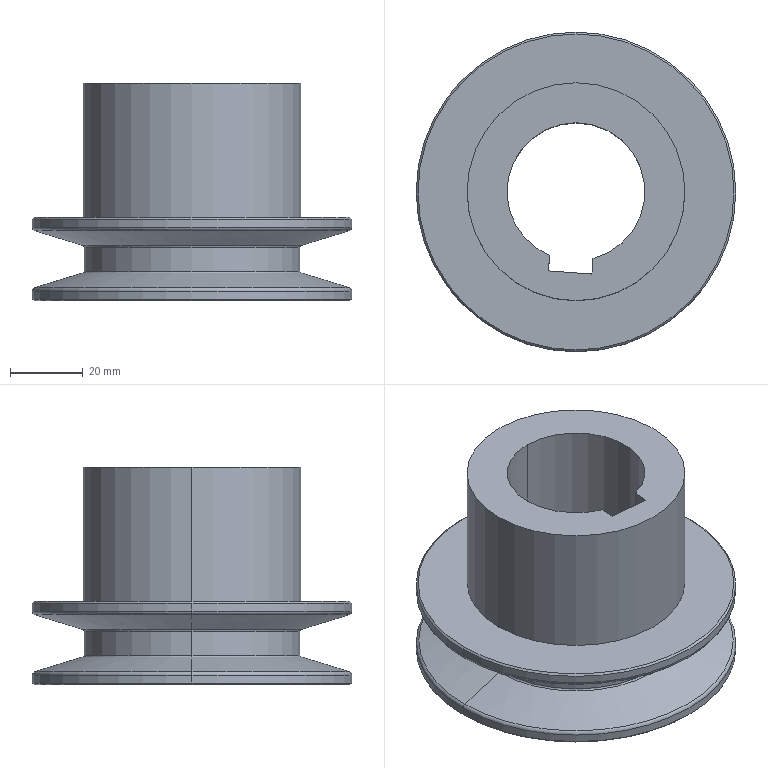Part | SolidWorks | features Fillet 2, ICE 2, Chamfer 1, RevCut 1, Revolution 1 | 1 solid | 32 faces | box 88 x 88 x 60 mm | volume 133834 mm3 | cylinder 10 | torus 8 | cone 8 | plane 6 | commonest cylinder face diameters 88 x4 38 x2 59.4 x2 60 x2
STEP:
#1=CARTESIAN_POINT('',(619.523,22.744,-118.047));
#2=VERTEX_POINT('',#1);
#3=CARTESIAN_POINT('',(532.938,22.744,-118.047));
#4=VERTEX_POINT('',#3);
#5=CARTESIAN_POINT('',(576.231,22.744,-118.047));
#6=DIRECTION('',(0.,0.,1.));
#7=DIRECTION('',(1.,0.,0.));
#8=AXIS2_PLACEMENT_3D('',#5,#6,#7);
#9=CIRCLE('',#8,43.292);
#10=EDGE_CURVE('',#2,#4,#9,.T.);
#11=ORIENTED_EDGE('',*,*,#10,.F.);
#12=CARTESIAN_POINT('',(620.231,22.744,-119.003));
#13=VERTEX_POINT('',#12);
#14=CARTESIAN_POINT('',(619.231,22.744,-119.003));
#15=DIRECTION('',(0.,1.,0.));
#16=DIRECTION('',(-1.,0.,0.));
#17=AXIS2_PLACEMENT_3D('',#14,#15,#16);
#18=CIRCLE('',#17,1.);
#19=EDGE_CURVE('',#2,#13,#18,.T.);
#20=ORIENTED_EDGE('',*,*,#19,.T.);
#21=CARTESIAN_POINT('',(532.231,22.744,-119.003));
#22=VERTEX_POINT('',#21);
#23=CARTESIAN_POINT('',(576.231,22.744,-119.003));
#24=DIRECTION('',(0.,0.,-1.));
#25=DIRECTION('',(-1.,0.,0.));
#26=AXIS2_PLACEMENT_3D('',#23,#24,#25);
#27=CIRCLE('',#26,44.);
#28=EDGE_CURVE('',#22,#13,#27,.T.);
#29=ORIENTED_EDGE('',*,*,#28,.F.);
#30=CARTESIAN_POINT('',(533.231,22.744,-119.003));
#31=DIRECTION('',(0.,-1.,0.));
#32=DIRECTION('',(0.,0.,-1.));
#33=AXIS2_PLACEMENT_3D('',#30,#31,#32);
#34=CIRCLE('',#33,1.);
#35=EDGE_CURVE('',#4,#22,#34,.T.);
#36=ORIENTED_EDGE('',*,*,#35,.F.);
#37=EDGE_LOOP('',(#11,#20,#29,#36));
#38=FACE_OUTER_BOUND('',#37,.T.);
#39=CARTESIAN_POINT('',(576.231,22.744,-119.003));
#40=DIRECTION('',(0.,0.,-1.));
#41=DIRECTION('',(-1.,0.,0.));
#42=AXIS2_PLACEMENT_3D('',#39,#40,#41);
#43=TOROIDAL_SURFACE('',#42,43.,1.);
#44=ADVANCED_FACE('',(#38),#43,.T.);
#45=CARTESIAN_POINT('',(620.231,22.744,-101.383));
#46=VERTEX_POINT('',#45);
#47=CARTESIAN_POINT('',(532.231,22.744,-101.383));
#48=VERTEX_POINT('',#47);
#49=CARTESIAN_POINT('',(576.231,22.744,-101.383));
#50=DIRECTION('',(0.,0.,1.));
#51=DIRECTION('',(-1.,0.,0.));
#52=AXIS2_PLACEMENT_3D('',#49,#50,#51);
#53=CIRCLE('',#52,44.);
#54=EDGE_CURVE('',#46,#48,#53,.T.);
#55=ORIENTED_EDGE('',*,*,#54,.F.);
#56=CARTESIAN_POINT('',(619.523,22.744,-102.339));
#57=VERTEX_POINT('',#56);
#58=CARTESIAN_POINT('',(619.231,22.744,-101.383));
#59=DIRECTION('',(0.,1.,0.));
#60=DIRECTION('',(-1.,0.,0.));
#61=AXIS2_PLACEMENT_3D('',#58,#59,#60);
#62=CIRCLE('',#61,1.);
#63=EDGE_CURVE('',#46,#57,#62,.T.);
#64=ORIENTED_EDGE('',*,*,#63,.T.);
#65=CARTESIAN_POINT('',(532.938,22.744,-102.339));
#66=VERTEX_POINT('',#65);
#67=CARTESIAN_POINT('',(576.231,22.744,-102.339));
#68=DIRECTION('',(0.,0.,-1.));
#69=DIRECTION('',(-1.,0.,0.));
#70=AXIS2_PLACEMENT_3D('',#67,#68,#69);
#71=CIRCLE('',#70,43.292);
#72=EDGE_CURVE('',#66,#57,#71,.T.);
#73=ORIENTED_EDGE('',*,*,#72,.F.);
#74=CARTESIAN_POINT('',(533.231,22.744,-101.383));
#75=DIRECTION('',(0.,-1.,0.));
#76=DIRECTION('',(0.,0.,-1.));
#77=AXIS2_PLACEMENT_3D('',#74,#75,#76);
#78=CIRCLE('',#77,1.);
#79=EDGE_CURVE('',#48,#66,#78,.T.);
#80=ORIENTED_EDGE('',*,*,#79,.F.);
#81=EDGE_LOOP('',(#55,#64,#73,#80));
#82=FACE_OUTER_BOUND('',#81,.T.);
#83=CARTESIAN_POINT('',(576.231,22.744,-101.383));
#84=DIRECTION('',(0.,0.,-1.));
#85=DIRECTION('',(-1.,0.,0.));
#86=AXIS2_PLACEMENT_3D('',#83,#84,#85);
#87=TOROIDAL_SURFACE('',#86,43.,1.);
#88=ADVANCED_FACE('',(#82),#87,.T.);
#89=CARTESIAN_POINT('',(546.531,22.744,-113.521));
#90=VERTEX_POINT('',#89);
#91=CARTESIAN_POINT('',(605.931,22.744,-113.521));
#92=VERTEX_POINT('',#91);
#93=CARTESIAN_POINT('',(576.231,22.744,-113.521));
#94=DIRECTION('',(0.,0.,1.));
#95=DIRECTION('',(1.,0.,0.));
#96=AXIS2_PLACEMENT_3D('',#93,#94,#95);
#97=CIRCLE('',#96,29.7);
#98=EDGE_CURVE('',#90,#92,#97,.T.);
#99=ORIENTED_EDGE('',*,*,#98,.F.);
#100=CARTESIAN_POINT('',(546.177,22.744,-113.999));
#101=VERTEX_POINT('',#100);
#102=CARTESIAN_POINT('',(546.031,22.744,-113.521));
#103=DIRECTION('',(0.,1.,0.));
#104=DIRECTION('',(-1.,0.,0.));
#105=AXIS2_PLACEMENT_3D('',#102,#103,#104);
#106=CIRCLE('',#105,0.5);
#107=EDGE_CURVE('',#90,#101,#106,.T.);
#108=ORIENTED_EDGE('',*,*,#107,.T.);
#109=CARTESIAN_POINT('',(606.284,22.744,-113.999));
#110=VERTEX_POINT('',#109);
#111=CARTESIAN_POINT('',(576.231,22.744,-113.999));
#112=DIRECTION('',(0.,0.,-1.));
#113=DIRECTION('',(-1.,0.,0.));
#114=AXIS2_PLACEMENT_3D('',#111,#112,#113);
#115=CIRCLE('',#114,30.054);
#116=EDGE_CURVE('',#110,#101,#115,.T.);
#117=ORIENTED_EDGE('',*,*,#116,.F.);
#118=CARTESIAN_POINT('',(606.431,22.744,-113.521));
#119=DIRECTION('',(0.,-1.,0.));
#120=DIRECTION('',(0.,0.,-1.));
#121=AXIS2_PLACEMENT_3D('',#118,#119,#120);
#122=CIRCLE('',#121,0.5);
#123=EDGE_CURVE('',#92,#110,#122,.T.);
#124=ORIENTED_EDGE('',*,*,#123,.F.);
#125=EDGE_LOOP('',(#99,#108,#117,#124));
#126=FACE_OUTER_BOUND('',#125,.T.);
#127=CARTESIAN_POINT('',(576.231,22.744,-113.521));
#128=DIRECTION('',(0.,0.,1.));
#129=DIRECTION('',(1.,0.,0.));
#130=AXIS2_PLACEMENT_3D('',#127,#128,#129);
#131=TOROIDAL_SURFACE('',#130,30.2,0.5);
#132=ADVANCED_FACE('',(#126),#131,.F.);
#133=CARTESIAN_POINT('',(546.177,22.744,-106.387));
#134=VERTEX_POINT('',#133);
#135=CARTESIAN_POINT('',(606.284,22.744,-106.387));
#136=VERTEX_POINT('',#135);
#137=CARTESIAN_POINT('',(576.231,22.744,-106.387));
#138=DIRECTION('',(0.,0.,1.));
#139=DIRECTION('',(1.,0.,0.));
#140=AXIS2_PLACEMENT_3D('',#137,#138,#139);
#141=CIRCLE('',#140,30.054);
#142=EDGE_CURVE('',#134,#136,#141,.T.);
#143=ORIENTED_EDGE('',*,*,#142,.F.);
#144=CARTESIAN_POINT('',(546.531,22.744,-106.865));
#145=VERTEX_POINT('',#144);
#146=CARTESIAN_POINT('',(546.031,22.744,-106.865));
#147=DIRECTION('',(0.,1.,0.));
#148=DIRECTION('',(-1.,0.,0.));
#149=AXIS2_PLACEMENT_3D('',#146,#147,#148);
#150=CIRCLE('',#149,0.5);
#151=EDGE_CURVE('',#134,#145,#150,.T.);
#152=ORIENTED_EDGE('',*,*,#151,.T.);
#153=CARTESIAN_POINT('',(605.931,22.744,-106.865));
#154=VERTEX_POINT('',#153);
#155=CARTESIAN_POINT('',(576.231,22.744,-106.865));
#156=DIRECTION('',(0.,0.,-1.));
#157=DIRECTION('',(1.,0.,0.));
#158=AXIS2_PLACEMENT_3D('',#155,#156,#157);
#159=CIRCLE('',#158,29.7);
#160=EDGE_CURVE('',#154,#145,#159,.T.);
#161=ORIENTED_EDGE('',*,*,#160,.F.);
#162=CARTESIAN_POINT('',(606.431,22.744,-106.865));
#163=DIRECTION('',(0.,-1.,0.));
#164=DIRECTION('',(0.,0.,-1.));
#165=AXIS2_PLACEMENT_3D('',#162,#163,#164);
#166=CIRCLE('',#165,0.5);
#167=EDGE_CURVE('',#136,#154,#166,.T.);
#168=ORIENTED_EDGE('',*,*,#167,.F.);
#169=EDGE_LOOP('',(#143,#152,#161,#168));
#170=FACE_OUTER_BOUND('',#169,.T.);
#171=CARTESIAN_POINT('',(576.231,22.744,-106.865));
#172=DIRECTION('',(0.,0.,1.));
#173=DIRECTION('',(1.,0.,0.));
#174=AXIS2_PLACEMENT_3D('',#171,#172,#173);
#175=TOROIDAL_SURFACE('',#174,30.2,0.5);
#176=ADVANCED_FACE('',(#170),#175,.F.);
#177=CARTESIAN_POINT('',(532.731,22.744,-121.693));
#178=VERTEX_POINT('',#177);
#179=CARTESIAN_POINT('',(619.731,22.744,-121.693));
#180=VERTEX_POINT('',#179);
#181=CARTESIAN_POINT('',(576.231,22.744,-121.693));
#182=DIRECTION('',(0.,0.,-1.));
#183=DIRECTION('',(-1.,0.,0.));
#184=AXIS2_PLACEMENT_3D('',#181,#182,#183);
#185=CIRCLE('',#184,43.5);
#186=EDGE_CURVE('',#178,#180,#185,.T.);
#187=ORIENTED_EDGE('',*,*,#186,.F.);
#188=CARTESIAN_POINT('',(532.231,22.744,-121.193));
#189=VERTEX_POINT('',#188);
#190=CARTESIAN_POINT('',(532.231,22.744,-121.193));
#191=DIRECTION('',(-0.7071,0.,0.7071));
#192=VECTOR('',#191,1000.);
#193=LINE('',#190,#192);
#194=EDGE_CURVE('',#178,#189,#193,.T.);
#195=ORIENTED_EDGE('',*,*,#194,.T.);
#196=CARTESIAN_POINT('',(620.231,22.744,-121.193));
#197=VERTEX_POINT('',#196);
#198=CARTESIAN_POINT('',(576.231,22.744,-121.193));
#199=DIRECTION('',(0.,0.,1.));
#200=DIRECTION('',(-1.,0.,0.));
#201=AXIS2_PLACEMENT_3D('',#198,#199,#200);
#202=CIRCLE('',#201,44.);
#203=EDGE_CURVE('',#197,#189,#202,.T.);
#204=ORIENTED_EDGE('',*,*,#203,.F.);
#205=CARTESIAN_POINT('',(620.231,22.744,-121.193));
#206=DIRECTION('',(0.7071,0.,0.7071));
#207=VECTOR('',#206,1000.);
#208=LINE('',#205,#207);
#209=EDGE_CURVE('',#180,#197,#208,.T.);
#210=ORIENTED_EDGE('',*,*,#209,.F.);
#211=EDGE_LOOP('',(#187,#195,#204,#210));
#212=FACE_OUTER_BOUND('',#211,.T.);
#213=CARTESIAN_POINT('',(576.231,22.744,-121.193));
#214=DIRECTION('',(0.,0.,1.));
#215=DIRECTION('',(1.,0.,0.));
#216=AXIS2_PLACEMENT_3D('',#213,#214,#215);
#217=CONICAL_SURFACE('',#216,44.,0.7854);
#218=ADVANCED_FACE('',(#212),#217,.T.);
#219=CARTESIAN_POINT('',(619.731,22.744,-98.693));
#220=VERTEX_POINT('',#219);
#221=CARTESIAN_POINT('',(532.731,22.744,-98.693));
#222=VERTEX_POINT('',#221);
#223=CARTESIAN_POINT('',(576.231,22.744,-98.693));
#224=DIRECTION('',(0.,0.,1.));
#225=DIRECTION('',(1.,0.,0.));
#226=AXIS2_PLACEMENT_3D('',#223,#224,#225);
#227=CIRCLE('',#226,43.5);
#228=EDGE_CURVE('',#220,#222,#227,.T.);
#229=ORIENTED_EDGE('',*,*,#228,.F.);
#230=CARTESIAN_POINT('',(620.231,22.744,-99.193));
#231=VERTEX_POINT('',#230);
#232=CARTESIAN_POINT('',(619.731,22.744,-98.693));
#233=DIRECTION('',(0.7071,0.,-0.7071));
#234=VECTOR('',#233,1000.);
#235=LINE('',#232,#234);
#236=EDGE_CURVE('',#220,#231,#235,.T.);
#237=ORIENTED_EDGE('',*,*,#236,.T.);
#238=CARTESIAN_POINT('',(532.231,22.744,-99.193));
#239=VERTEX_POINT('',#238);
#240=CARTESIAN_POINT('',(576.231,22.744,-99.193));
#241=DIRECTION('',(0.,0.,-1.));
#242=DIRECTION('',(1.,0.,0.));
#243=AXIS2_PLACEMENT_3D('',#240,#241,#242);
#244=CIRCLE('',#243,44.);
#245=EDGE_CURVE('',#239,#231,#244,.T.);
#246=ORIENTED_EDGE('',*,*,#245,.F.);
#247=CARTESIAN_POINT('',(532.731,22.744,-98.693));
#248=DIRECTION('',(-0.7071,0.,-0.7071));
#249=VECTOR('',#248,1000.);
#250=LINE('',#247,#249);
#251=EDGE_CURVE('',#222,#239,#250,.T.);
#252=ORIENTED_EDGE('',*,*,#251,.F.);
#253=EDGE_LOOP('',(#229,#237,#246,#252));
#254=FACE_OUTER_BOUND('',#253,.T.);
#255=CARTESIAN_POINT('',(576.231,22.744,-98.693));
#256=DIRECTION('',(0.,0.,-1.));
#257=DIRECTION('',(-1.,0.,0.));
#258=AXIS2_PLACEMENT_3D('',#255,#256,#257);
#259=CONICAL_SURFACE('',#258,43.5,0.7854);
#260=ADVANCED_FACE('',(#254),#259,.T.);
#261=CARTESIAN_POINT('',(576.231,41.744,-61.693));
#262=VERTEX_POINT('',#261);
#263=CARTESIAN_POINT('',(580.912,4.33,-61.693));
#264=VERTEX_POINT('',#263);
#265=CARTESIAN_POINT('',(576.231,22.744,-61.693));
#266=DIRECTION('',(0.,0.,-1.));
#267=DIRECTION('',(0.,1.,0.));
#268=AXIS2_PLACEMENT_3D('',#265,#266,#267);
#269=CIRCLE('',#268,19.);
#270=EDGE_CURVE('',#262,#264,#269,.T.);
#271=ORIENTED_EDGE('',*,*,#270,.F.);
#272=CARTESIAN_POINT('',(576.231,41.744,-121.693));
#273=VERTEX_POINT('',#272);
#274=CARTESIAN_POINT('',(576.231,41.744,-61.693));
#275=DIRECTION('',(0.,0.,-1.));
#276=VECTOR('',#275,1000.);
#277=LINE('',#274,#276);
#278=EDGE_CURVE('',#262,#273,#277,.T.);
#279=ORIENTED_EDGE('',*,*,#278,.T.);
#280=CARTESIAN_POINT('',(580.912,4.33,-121.693));
#281=VERTEX_POINT('',#280);
#282=CARTESIAN_POINT('',(576.231,22.744,-121.693));
#283=DIRECTION('',(0.,0.,-1.));
#284=DIRECTION('',(0.,1.,0.));
#285=AXIS2_PLACEMENT_3D('',#282,#283,#284);
#286=CIRCLE('',#285,19.);
#287=EDGE_CURVE('',#273,#281,#286,.T.);
#288=ORIENTED_EDGE('',*,*,#287,.T.);
#289=CARTESIAN_POINT('',(580.912,4.33,-61.693));
#290=DIRECTION('',(0.,0.,-1.));
#291=VECTOR('',#290,1000.);
#292=LINE('',#289,#291);
#293=EDGE_CURVE('',#264,#281,#292,.T.);
#294=ORIENTED_EDGE('',*,*,#293,.F.);
#295=EDGE_LOOP('',(#271,#279,#288,#294));
#296=FACE_OUTER_BOUND('',#295,.T.);
#297=CARTESIAN_POINT('',(576.231,22.744,-61.693));
#298=DIRECTION('',(0.,0.,-1.));
#299=DIRECTION('',(0.,1.,0.));
#300=AXIS2_PLACEMENT_3D('',#297,#298,#299);
#301=CYLINDRICAL_SURFACE('',#300,19.);
#302=ADVANCED_FACE('',(#296),#301,.F.);
#303=CARTESIAN_POINT('',(606.231,22.744,-61.693));
#304=VERTEX_POINT('',#303);
#305=CARTESIAN_POINT('',(546.231,22.744,-61.693));
#306=VERTEX_POINT('',#305);
#307=CARTESIAN_POINT('',(576.231,22.744,-61.693));
#308=DIRECTION('',(0.,0.,1.));
#309=DIRECTION('',(1.,0.,0.));
#310=AXIS2_PLACEMENT_3D('',#307,#308,#309);
#311=CIRCLE('',#310,30.);
#312=EDGE_CURVE('',#304,#306,#311,.T.);
#313=ORIENTED_EDGE('',*,*,#312,.F.);
#314=CARTESIAN_POINT('',(606.231,22.744,-98.693));
#315=VERTEX_POINT('',#314);
#316=CARTESIAN_POINT('',(606.231,22.744,-61.693));
#317=DIRECTION('',(0.,0.,-1.));
#318=VECTOR('',#317,1000.);
#319=LINE('',#316,#318);
#320=EDGE_CURVE('',#304,#315,#319,.T.);
#321=ORIENTED_EDGE('',*,*,#320,.T.);
#322=CARTESIAN_POINT('',(546.231,22.744,-98.693));
#323=VERTEX_POINT('',#322);
#324=CARTESIAN_POINT('',(576.231,22.744,-98.693));
#325=DIRECTION('',(0.,0.,1.));
#326=DIRECTION('',(1.,0.,0.));
#327=AXIS2_PLACEMENT_3D('',#324,#325,#326);
#328=CIRCLE('',#327,30.);
#329=EDGE_CURVE('',#315,#323,#328,.T.);
#330=ORIENTED_EDGE('',*,*,#329,.T.);
#331=CARTESIAN_POINT('',(546.231,22.744,-61.693));
#332=DIRECTION('',(0.,0.,-1.));
#333=VECTOR('',#332,1000.);
#334=LINE('',#331,#333);
#335=EDGE_CURVE('',#306,#323,#334,.T.);
#336=ORIENTED_EDGE('',*,*,#335,.F.);
#337=EDGE_LOOP('',(#313,#321,#330,#336));
#338=FACE_OUTER_BOUND('',#337,.T.);
#339=CARTESIAN_POINT('',(576.231,22.744,-61.693));
#340=DIRECTION('',(0.,0.,-1.));
#341=DIRECTION('',(-1.,0.,0.));
#342=AXIS2_PLACEMENT_3D('',#339,#340,#341);
#343=CYLINDRICAL_SURFACE('',#342,30.);
#344=ADVANCED_FACE('',(#338),#343,.T.);
#345=CARTESIAN_POINT('',(576.231,22.744,-113.999));
#346=DIRECTION('',(0.,0.,-1.));
#347=DIRECTION('',(-1.,0.,0.));
#348=AXIS2_PLACEMENT_3D('',#345,#346,#347);
#349=CIRCLE('',#348,30.054);
#350=EDGE_CURVE('',#101,#110,#349,.T.);
#351=ORIENTED_EDGE('',*,*,#350,.T.);
#352=CARTESIAN_POINT('',(605.931,22.744,-113.891));
#353=DIRECTION('',(0.9563,0.,-0.2924));
#354=VECTOR('',#353,1000.);
#355=LINE('',#352,#354);
#356=EDGE_CURVE('',#110,#2,#355,.T.);
#357=ORIENTED_EDGE('',*,*,#356,.T.);
#358=ORIENTED_EDGE('',*,*,#10,.T.);
#359=CARTESIAN_POINT('',(546.531,22.744,-113.891));
#360=DIRECTION('',(-0.9563,0.,-0.2924));
#361=VECTOR('',#360,1000.);
#362=LINE('',#359,#361);
#363=EDGE_CURVE('',#101,#4,#362,.T.);
#364=ORIENTED_EDGE('',*,*,#363,.F.);
#365=EDGE_LOOP('',(#351,#357,#358,#364));
#366=FACE_OUTER_BOUND('',#365,.T.);
#367=CARTESIAN_POINT('',(576.231,22.744,-113.891));
#368=DIRECTION('',(0.,0.,-1.));
#369=DIRECTION('',(-1.,0.,0.));
#370=AXIS2_PLACEMENT_3D('',#367,#368,#369);
#371=CONICAL_SURFACE('',#370,29.7,1.274);
#372=ADVANCED_FACE('',(#366),#371,.T.);
#373=CARTESIAN_POINT('',(576.231,22.744,-113.521));
#374=DIRECTION('',(0.,0.,1.));
#375=DIRECTION('',(1.,0.,0.));
#376=AXIS2_PLACEMENT_3D('',#373,#374,#375);
#377=CIRCLE('',#376,29.7);
#378=EDGE_CURVE('',#92,#90,#377,.T.);
#379=ORIENTED_EDGE('',*,*,#378,.T.);
#380=CARTESIAN_POINT('',(546.531,22.744,-121.693));
#381=DIRECTION('',(0.,0.,1.));
#382=VECTOR('',#381,1000.);
#383=LINE('',#380,#382);
#384=EDGE_CURVE('',#90,#145,#383,.T.);
#385=ORIENTED_EDGE('',*,*,#384,.T.);
#386=CARTESIAN_POINT('',(576.231,22.744,-106.865));
#387=DIRECTION('',(0.,0.,-1.));
#388=DIRECTION('',(1.,0.,0.));
#389=AXIS2_PLACEMENT_3D('',#386,#387,#388);
#390=CIRCLE('',#389,29.7);
#391=EDGE_CURVE('',#145,#154,#390,.T.);
#392=ORIENTED_EDGE('',*,*,#391,.T.);
#393=CARTESIAN_POINT('',(605.931,22.744,-121.693));
#394=DIRECTION('',(0.,0.,1.));
#395=VECTOR('',#394,1000.);
#396=LINE('',#393,#395);
#397=EDGE_CURVE('',#92,#154,#396,.T.);
#398=ORIENTED_EDGE('',*,*,#397,.F.);
#399=EDGE_LOOP('',(#379,#385,#392,#398));
#400=FACE_OUTER_BOUND('',#399,.T.);
#401=CARTESIAN_POINT('',(576.231,22.744,-121.693));
#402=DIRECTION('',(0.,0.,1.));
#403=DIRECTION('',(1.,0.,0.));
#404=AXIS2_PLACEMENT_3D('',#401,#402,#403);
#405=CYLINDRICAL_SURFACE('',#404,29.7);
#406=ADVANCED_FACE('',(#400),#405,.T.);
#407=CARTESIAN_POINT('',(576.231,22.744,-106.387));
#408=DIRECTION('',(0.,0.,1.));
#409=DIRECTION('',(1.,0.,0.));
#410=AXIS2_PLACEMENT_3D('',#407,#408,#409);
#411=CIRCLE('',#410,30.054);
#412=EDGE_CURVE('',#136,#134,#411,.T.);
#413=ORIENTED_EDGE('',*,*,#412,.T.);
#414=CARTESIAN_POINT('',(532.231,22.744,-102.123));
#415=DIRECTION('',(-0.9563,0.,0.2924));
#416=VECTOR('',#415,1000.);
#417=LINE('',#414,#416);
#418=EDGE_CURVE('',#134,#66,#417,.T.);
#419=ORIENTED_EDGE('',*,*,#418,.T.);
#420=ORIENTED_EDGE('',*,*,#72,.T.);
#421=CARTESIAN_POINT('',(620.231,22.744,-102.123));
#422=DIRECTION('',(0.9563,0.,0.2924));
#423=VECTOR('',#422,1000.);
#424=LINE('',#421,#423);
#425=EDGE_CURVE('',#136,#57,#424,.T.);
#426=ORIENTED_EDGE('',*,*,#425,.F.);
#427=EDGE_LOOP('',(#413,#419,#420,#426));
#428=FACE_OUTER_BOUND('',#427,.T.);
#429=CARTESIAN_POINT('',(576.231,22.744,-102.123));
#430=DIRECTION('',(0.,0.,1.));
#431=DIRECTION('',(1.,0.,0.));
#432=AXIS2_PLACEMENT_3D('',#429,#430,#431);
#433=CONICAL_SURFACE('',#432,44.,1.274);
#434=ADVANCED_FACE('',(#428),#433,.T.);
#435=ORIENTED_EDGE('',*,*,#54,.T.);
#436=CARTESIAN_POINT('',(532.231,22.744,-121.693));
#437=DIRECTION('',(0.,0.,1.));
#438=VECTOR('',#437,1000.);
#439=LINE('',#436,#438);
#440=EDGE_CURVE('',#48,#239,#439,.T.);
#441=ORIENTED_EDGE('',*,*,#440,.T.);
#442=ORIENTED_EDGE('',*,*,#245,.T.);
#443=CARTESIAN_POINT('',(620.231,22.744,-121.693));
#444=DIRECTION('',(0.,0.,1.));
#445=VECTOR('',#444,1000.);
#446=LINE('',#443,#445);
#447=EDGE_CURVE('',#46,#231,#446,.T.);
#448=ORIENTED_EDGE('',*,*,#447,.F.);
#449=EDGE_LOOP('',(#435,#441,#442,#448));
#450=FACE_OUTER_BOUND('',#449,.T.);
#451=CARTESIAN_POINT('',(576.231,22.744,-121.693));
#452=DIRECTION('',(0.,0.,1.));
#453=DIRECTION('',(1.,0.,0.));
#454=AXIS2_PLACEMENT_3D('',#451,#452,#453);
#455=CYLINDRICAL_SURFACE('',#454,44.);
#456=ADVANCED_FACE('',(#450),#455,.T.);
#457=ORIENTED_EDGE('',*,*,#203,.T.);
#458=CARTESIAN_POINT('',(532.231,22.744,-121.693));
#459=DIRECTION('',(0.,0.,1.));
#460=VECTOR('',#459,1000.);
#461=LINE('',#458,#460);
#462=EDGE_CURVE('',#189,#22,#461,.T.);
#463=ORIENTED_EDGE('',*,*,#462,.T.);
#464=ORIENTED_EDGE('',*,*,#28,.T.);
#465=CARTESIAN_POINT('',(620.231,22.744,-121.693));
#466=DIRECTION('',(0.,0.,1.));
#467=VECTOR('',#466,1000.);
#468=LINE('',#465,#467);
#469=EDGE_CURVE('',#197,#13,#468,.T.);
#470=ORIENTED_EDGE('',*,*,#469,.F.);
#471=EDGE_LOOP('',(#457,#463,#464,#470));
#472=FACE_OUTER_BOUND('',#471,.T.);
#473=CARTESIAN_POINT('',(576.231,22.744,-121.693));
#474=DIRECTION('',(0.,0.,1.));
#475=DIRECTION('',(1.,0.,0.));
#476=AXIS2_PLACEMENT_3D('',#473,#474,#475);
#477=CYLINDRICAL_SURFACE('',#476,44.);
#478=ADVANCED_FACE('',(#472),#477,.T.);
#479=ORIENTED_EDGE('',*,*,#462,.F.);
#480=CARTESIAN_POINT('',(576.231,22.744,-121.193));
#481=DIRECTION('',(0.,0.,1.));
#482=DIRECTION('',(-1.,0.,0.));
#483=AXIS2_PLACEMENT_3D('',#480,#481,#482);
#484=CIRCLE('',#483,44.);
#485=EDGE_CURVE('',#189,#197,#484,.T.);
#486=ORIENTED_EDGE('',*,*,#485,.T.);
#487=ORIENTED_EDGE('',*,*,#469,.T.);
#488=CARTESIAN_POINT('',(576.231,22.744,-119.003));
#489=DIRECTION('',(0.,0.,-1.));
#490=DIRECTION('',(-1.,0.,0.));
#491=AXIS2_PLACEMENT_3D('',#488,#489,#490);
#492=CIRCLE('',#491,44.);
#493=EDGE_CURVE('',#13,#22,#492,.T.);
#494=ORIENTED_EDGE('',*,*,#493,.T.);
#495=EDGE_LOOP('',(#479,#486,#487,#494));
#496=FACE_OUTER_BOUND('',#495,.T.);
#497=CARTESIAN_POINT('',(576.231,22.744,-121.693));
#498=DIRECTION('',(0.,0.,1.));
#499=DIRECTION('',(1.,0.,0.));
#500=AXIS2_PLACEMENT_3D('',#497,#498,#499);
#501=CYLINDRICAL_SURFACE('',#500,44.);
#502=ADVANCED_FACE('',(#496),#501,.T.);
#503=CARTESIAN_POINT('',(576.231,22.744,-121.693));
#504=DIRECTION('',(0.,0.,-1.));
#505=DIRECTION('',(-1.,0.,0.));
#506=AXIS2_PLACEMENT_3D('',#503,#504,#505);
#507=CIRCLE('',#506,43.5);
#508=EDGE_CURVE('',#180,#178,#507,.T.);
#509=ORIENTED_EDGE('',*,*,#508,.T.);
#510=ORIENTED_EDGE('',*,*,#186,.T.);
#511=EDGE_LOOP('',(#509,#510));
#512=FACE_OUTER_BOUND('',#511,.T.);
#513=CARTESIAN_POINT('',(568.943,5.197,-121.693));
#514=VERTEX_POINT('',#513);
#515=CARTESIAN_POINT('',(576.231,22.744,-121.693));
#516=DIRECTION('',(0.,0.,-1.));
#517=DIRECTION('',(0.,1.,0.));
#518=AXIS2_PLACEMENT_3D('',#515,#516,#517);
#519=CIRCLE('',#518,19.);
#520=EDGE_CURVE('',#514,#273,#519,.T.);
#521=ORIENTED_EDGE('',*,*,#520,.F.);
#522=CARTESIAN_POINT('',(568.634,0.9361,-121.693));
#523=VERTEX_POINT('',#522);
#524=CARTESIAN_POINT('',(568.634,0.9361,-121.693));
#525=DIRECTION('',(0.07229,0.9974,0.));
#526=VECTOR('',#525,1000.);
#527=LINE('',#524,#526);
#528=EDGE_CURVE('',#523,#514,#527,.T.);
#529=ORIENTED_EDGE('',*,*,#528,.F.);
#530=CARTESIAN_POINT('',(580.603,0.06857,-121.693));
#531=VERTEX_POINT('',#530);
#532=CARTESIAN_POINT('',(580.603,0.06857,-121.693));
#533=DIRECTION('',(-0.9974,0.07229,0.));
#534=VECTOR('',#533,1000.);
#535=LINE('',#532,#534);
#536=EDGE_CURVE('',#531,#523,#535,.T.);
#537=ORIENTED_EDGE('',*,*,#536,.F.);
#538=CARTESIAN_POINT('',(580.912,4.33,-121.693));
#539=DIRECTION('',(-0.07229,-0.9974,0.));
#540=VECTOR('',#539,1000.);
#541=LINE('',#538,#540);
#542=EDGE_CURVE('',#281,#531,#541,.T.);
#543=ORIENTED_EDGE('',*,*,#542,.F.);
#544=ORIENTED_EDGE('',*,*,#287,.F.);
#545=EDGE_LOOP('',(#521,#529,#537,#543,#544));
#546=FACE_BOUND('',#545,.T.);
#547=CARTESIAN_POINT('',(620.231,22.744,-121.693));
#548=DIRECTION('',(0.,0.,-1.));
#549=DIRECTION('',(-1.,0.,0.));
#550=AXIS2_PLACEMENT_3D('',#547,#548,#549);
#551=PLANE('',#550);
#552=ADVANCED_FACE('',(#512,#546),#551,.T.);
#553=CARTESIAN_POINT('',(576.231,22.744,-98.693));
#554=DIRECTION('',(0.,0.,1.));
#555=DIRECTION('',(1.,0.,0.));
#556=AXIS2_PLACEMENT_3D('',#553,#554,#555);
#557=CIRCLE('',#556,43.5);
#558=EDGE_CURVE('',#222,#220,#557,.T.);
#559=ORIENTED_EDGE('',*,*,#558,.T.);
#560=ORIENTED_EDGE('',*,*,#228,.T.);
#561=EDGE_LOOP('',(#559,#560));
#562=FACE_OUTER_BOUND('',#561,.T.);
#563=CARTESIAN_POINT('',(576.231,22.744,-98.693));
#564=DIRECTION('',(0.,0.,1.));
#565=DIRECTION('',(1.,0.,0.));
#566=AXIS2_PLACEMENT_3D('',#563,#564,#565);
#567=CIRCLE('',#566,30.);
#568=EDGE_CURVE('',#323,#315,#567,.T.);
#569=ORIENTED_EDGE('',*,*,#568,.F.);
#570=ORIENTED_EDGE('',*,*,#329,.F.);
#571=EDGE_LOOP('',(#569,#570));
#572=FACE_BOUND('',#571,.T.);
#573=CARTESIAN_POINT('',(576.231,22.744,-98.693));
#574=DIRECTION('',(0.,0.,1.));
#575=DIRECTION('',(1.,0.,0.));
#576=AXIS2_PLACEMENT_3D('',#573,#574,#575);
#577=PLANE('',#576);
#578=ADVANCED_FACE('',(#562,#572),#577,.T.);
#579=ORIENTED_EDGE('',*,*,#440,.F.);
#580=CARTESIAN_POINT('',(576.231,22.744,-101.383));
#581=DIRECTION('',(0.,0.,1.));
#582=DIRECTION('',(-1.,0.,0.));
#583=AXIS2_PLACEMENT_3D('',#580,#581,#582);
#584=CIRCLE('',#583,44.);
#585=EDGE_CURVE('',#48,#46,#584,.T.);
#586=ORIENTED_EDGE('',*,*,#585,.T.);
#587=ORIENTED_EDGE('',*,*,#447,.T.);
#588=CARTESIAN_POINT('',(576.231,22.744,-99.193));
#589=DIRECTION('',(0.,0.,-1.));
#590=DIRECTION('',(1.,0.,0.));
#591=AXIS2_PLACEMENT_3D('',#588,#589,#590);
#592=CIRCLE('',#591,44.);
#593=EDGE_CURVE('',#231,#239,#592,.T.);
#594=ORIENTED_EDGE('',*,*,#593,.T.);
#595=EDGE_LOOP('',(#579,#586,#587,#594));
#596=FACE_OUTER_BOUND('',#595,.T.);
#597=CARTESIAN_POINT('',(576.231,22.744,-121.693));
#598=DIRECTION('',(0.,0.,1.));
#599=DIRECTION('',(1.,0.,0.));
#600=AXIS2_PLACEMENT_3D('',#597,#598,#599);
#601=CYLINDRICAL_SURFACE('',#600,44.);
#602=ADVANCED_FACE('',(#596),#601,.T.);
#603=ORIENTED_EDGE('',*,*,#418,.F.);
#604=ORIENTED_EDGE('',*,*,#142,.T.);
#605=ORIENTED_EDGE('',*,*,#425,.T.);
#606=CARTESIAN_POINT('',(576.231,22.744,-102.339));
#607=DIRECTION('',(0.,0.,-1.));
#608=DIRECTION('',(-1.,0.,0.));
#609=AXIS2_PLACEMENT_3D('',#606,#607,#608);
#610=CIRCLE('',#609,43.292);
#611=EDGE_CURVE('',#57,#66,#610,.T.);
#612=ORIENTED_EDGE('',*,*,#611,.T.);
#613=EDGE_LOOP('',(#603,#604,#605,#612));
#614=FACE_OUTER_BOUND('',#613,.T.);
#615=CARTESIAN_POINT('',(576.231,22.744,-102.123));
#616=DIRECTION('',(0.,0.,1.));
#617=DIRECTION('',(1.,0.,0.));
#618=AXIS2_PLACEMENT_3D('',#615,#616,#617);
#619=CONICAL_SURFACE('',#618,44.,1.274);
#620=ADVANCED_FACE('',(#614),#619,.T.);
#621=ORIENTED_EDGE('',*,*,#384,.F.);
#622=ORIENTED_EDGE('',*,*,#98,.T.);
#623=ORIENTED_EDGE('',*,*,#397,.T.);
#624=ORIENTED_EDGE('',*,*,#160,.T.);
#625=EDGE_LOOP('',(#621,#622,#623,#624));
#626=FACE_OUTER_BOUND('',#625,.T.);
#627=CARTESIAN_POINT('',(576.231,22.744,-121.693));
#628=DIRECTION('',(0.,0.,1.));
#629=DIRECTION('',(1.,0.,0.));
#630=AXIS2_PLACEMENT_3D('',#627,#628,#629);
#631=CYLINDRICAL_SURFACE('',#630,29.7);
#632=ADVANCED_FACE('',(#626),#631,.T.);
#633=ORIENTED_EDGE('',*,*,#356,.F.);
#634=ORIENTED_EDGE('',*,*,#116,.T.);
#635=ORIENTED_EDGE('',*,*,#363,.T.);
#636=CARTESIAN_POINT('',(576.231,22.744,-118.047));
#637=DIRECTION('',(0.,0.,1.));
#638=DIRECTION('',(1.,0.,0.));
#639=AXIS2_PLACEMENT_3D('',#636,#637,#638);
#640=CIRCLE('',#639,43.292);
#641=EDGE_CURVE('',#4,#2,#640,.T.);
#642=ORIENTED_EDGE('',*,*,#641,.T.);
#643=EDGE_LOOP('',(#633,#634,#635,#642));
#644=FACE_OUTER_BOUND('',#643,.T.);
#645=CARTESIAN_POINT('',(576.231,22.744,-113.891));
#646=DIRECTION('',(0.,0.,-1.));
#647=DIRECTION('',(-1.,0.,0.));
#648=AXIS2_PLACEMENT_3D('',#645,#646,#647);
#649=CONICAL_SURFACE('',#648,29.7,1.274);
#650=ADVANCED_FACE('',(#644),#649,.T.);
#651=ORIENTED_EDGE('',*,*,#320,.F.);
#652=CARTESIAN_POINT('',(576.231,22.744,-61.693));
#653=DIRECTION('',(0.,0.,1.));
#654=DIRECTION('',(1.,0.,0.));
#655=AXIS2_PLACEMENT_3D('',#652,#653,#654);
#656=CIRCLE('',#655,30.);
#657=EDGE_CURVE('',#306,#304,#656,.T.);
#658=ORIENTED_EDGE('',*,*,#657,.F.);
#659=ORIENTED_EDGE('',*,*,#335,.T.);
#660=ORIENTED_EDGE('',*,*,#568,.T.);
#661=EDGE_LOOP('',(#651,#658,#659,#660));
#662=FACE_OUTER_BOUND('',#661,.T.);
#663=CARTESIAN_POINT('',(576.231,22.744,-61.693));
#664=DIRECTION('',(0.,0.,-1.));
#665=DIRECTION('',(-1.,0.,0.));
#666=AXIS2_PLACEMENT_3D('',#663,#664,#665);
#667=CYLINDRICAL_SURFACE('',#666,30.);
#668=ADVANCED_FACE('',(#662),#667,.T.);
#669=CARTESIAN_POINT('',(568.943,5.197,-61.693));
#670=VERTEX_POINT('',#669);
#671=CARTESIAN_POINT('',(576.231,22.744,-61.693));
#672=DIRECTION('',(0.,0.,-1.));
#673=DIRECTION('',(0.,1.,0.));
#674=AXIS2_PLACEMENT_3D('',#671,#672,#673);
#675=CIRCLE('',#674,19.);
#676=EDGE_CURVE('',#670,#262,#675,.T.);
#677=ORIENTED_EDGE('',*,*,#676,.T.);
#678=ORIENTED_EDGE('',*,*,#270,.T.);
#679=CARTESIAN_POINT('',(580.603,0.06857,-61.693));
#680=VERTEX_POINT('',#679);
#681=CARTESIAN_POINT('',(580.912,4.33,-61.693));
#682=DIRECTION('',(-0.07229,-0.9974,0.));
#683=VECTOR('',#682,1000.);
#684=LINE('',#681,#683);
#685=EDGE_CURVE('',#264,#680,#684,.T.);
#686=ORIENTED_EDGE('',*,*,#685,.T.);
#687=CARTESIAN_POINT('',(568.634,0.9361,-61.693));
#688=VERTEX_POINT('',#687);
#689=CARTESIAN_POINT('',(580.603,0.06857,-61.693));
#690=DIRECTION('',(-0.9974,0.07229,0.));
#691=VECTOR('',#690,1000.);
#692=LINE('',#689,#691);
#693=EDGE_CURVE('',#680,#688,#692,.T.);
#694=ORIENTED_EDGE('',*,*,#693,.T.);
#695=CARTESIAN_POINT('',(568.634,0.9361,-61.693));
#696=DIRECTION('',(0.07229,0.9974,0.));
#697=VECTOR('',#696,1000.);
#698=LINE('',#695,#697);
#699=EDGE_CURVE('',#688,#670,#698,.T.);
#700=ORIENTED_EDGE('',*,*,#699,.T.);
#701=EDGE_LOOP('',(#677,#678,#686,#694,#700));
#702=FACE_BOUND('',#701,.T.);
#703=ORIENTED_EDGE('',*,*,#657,.T.);
#704=ORIENTED_EDGE('',*,*,#312,.T.);
#705=EDGE_LOOP('',(#703,#704));
#706=FACE_OUTER_BOUND('',#705,.T.);
#707=CARTESIAN_POINT('',(576.231,22.744,-61.693));
#708=DIRECTION('',(0.,0.,1.));
#709=DIRECTION('',(1.,0.,0.));
#710=AXIS2_PLACEMENT_3D('',#707,#708,#709);
#711=PLANE('',#710);
#712=ADVANCED_FACE('',(#702,#706),#711,.T.);
#713=ORIENTED_EDGE('',*,*,#542,.T.);
#714=CARTESIAN_POINT('',(580.603,0.06857,-61.693));
#715=DIRECTION('',(0.,0.,-1.));
#716=VECTOR('',#715,1000.);
#717=LINE('',#714,#716);
#718=EDGE_CURVE('',#680,#531,#717,.T.);
#719=ORIENTED_EDGE('',*,*,#718,.F.);
#720=ORIENTED_EDGE('',*,*,#685,.F.);
#721=ORIENTED_EDGE('',*,*,#293,.T.);
#722=EDGE_LOOP('',(#713,#719,#720,#721));
#723=FACE_OUTER_BOUND('',#722,.T.);
#724=CARTESIAN_POINT('',(580.912,4.33,-61.693));
#725=DIRECTION('',(0.9974,-0.07229,0.));
#726=DIRECTION('',(0.07229,0.9974,0.));
#727=AXIS2_PLACEMENT_3D('',#724,#725,#726);
#728=PLANE('',#727);
#729=ADVANCED_FACE('',(#723),#728,.F.);
#730=ORIENTED_EDGE('',*,*,#528,.T.);
#731=CARTESIAN_POINT('',(568.943,5.197,-61.693));
#732=DIRECTION('',(0.,0.,-1.));
#733=VECTOR('',#732,1000.);
#734=LINE('',#731,#733);
#735=EDGE_CURVE('',#670,#514,#734,.T.);
#736=ORIENTED_EDGE('',*,*,#735,.F.);
#737=ORIENTED_EDGE('',*,*,#699,.F.);
#738=CARTESIAN_POINT('',(568.634,0.9361,-61.693));
#739=DIRECTION('',(0.,0.,-1.));
#740=VECTOR('',#739,1000.);
#741=LINE('',#738,#740);
#742=EDGE_CURVE('',#688,#523,#741,.T.);
#743=ORIENTED_EDGE('',*,*,#742,.T.);
#744=EDGE_LOOP('',(#730,#736,#737,#743));
#745=FACE_OUTER_BOUND('',#744,.T.);
#746=CARTESIAN_POINT('',(568.634,0.9361,-61.693));
#747=DIRECTION('',(-0.9974,0.07229,0.));
#748=DIRECTION('',(-0.07229,-0.9974,0.));
#749=AXIS2_PLACEMENT_3D('',#746,#747,#748);
#750=PLANE('',#749);
#751=ADVANCED_FACE('',(#745),#750,.F.);
#752=ORIENTED_EDGE('',*,*,#536,.T.);
#753=ORIENTED_EDGE('',*,*,#742,.F.);
#754=ORIENTED_EDGE('',*,*,#693,.F.);
#755=ORIENTED_EDGE('',*,*,#718,.T.);
#756=EDGE_LOOP('',(#752,#753,#754,#755));
#757=FACE_OUTER_BOUND('',#756,.T.);
#758=CARTESIAN_POINT('',(580.603,0.06857,-61.693));
#759=DIRECTION('',(-0.07229,-0.9974,0.));
#760=DIRECTION('',(0.9974,-0.07229,0.));
#761=AXIS2_PLACEMENT_3D('',#758,#759,#760);
#762=PLANE('',#761);
#763=ADVANCED_FACE('',(#757),#762,.F.);
#764=ORIENTED_EDGE('',*,*,#278,.F.);
#765=ORIENTED_EDGE('',*,*,#676,.F.);
#766=ORIENTED_EDGE('',*,*,#735,.T.);
#767=ORIENTED_EDGE('',*,*,#520,.T.);
#768=EDGE_LOOP('',(#764,#765,#766,#767));
#769=FACE_OUTER_BOUND('',#768,.T.);
#770=CARTESIAN_POINT('',(576.231,22.744,-61.693));
#771=DIRECTION('',(0.,0.,-1.));
#772=DIRECTION('',(0.,1.,0.));
#773=AXIS2_PLACEMENT_3D('',#770,#771,#772);
#774=CYLINDRICAL_SURFACE('',#773,19.);
#775=ADVANCED_FACE('',(#769),#774,.F.);
#776=ORIENTED_EDGE('',*,*,#236,.F.);
#777=ORIENTED_EDGE('',*,*,#558,.F.);
#778=ORIENTED_EDGE('',*,*,#251,.T.);
#779=ORIENTED_EDGE('',*,*,#593,.F.);
#780=EDGE_LOOP('',(#776,#777,#778,#779));
#781=FACE_OUTER_BOUND('',#780,.T.);
#782=CARTESIAN_POINT('',(576.231,22.744,-98.693));
#783=DIRECTION('',(0.,0.,-1.));
#784=DIRECTION('',(-1.,0.,0.));
#785=AXIS2_PLACEMENT_3D('',#782,#783,#784);
#786=CONICAL_SURFACE('',#785,43.5,0.7854);
#787=ADVANCED_FACE('',(#781),#786,.T.);
#788=ORIENTED_EDGE('',*,*,#194,.F.);
#789=ORIENTED_EDGE('',*,*,#508,.F.);
#790=ORIENTED_EDGE('',*,*,#209,.T.);
#791=ORIENTED_EDGE('',*,*,#485,.F.);
#792=EDGE_LOOP('',(#788,#789,#790,#791));
#793=FACE_OUTER_BOUND('',#792,.T.);
#794=CARTESIAN_POINT('',(576.231,22.744,-121.193));
#795=DIRECTION('',(0.,0.,1.));
#796=DIRECTION('',(1.,0.,0.));
#797=AXIS2_PLACEMENT_3D('',#794,#795,#796);
#798=CONICAL_SURFACE('',#797,44.,0.7854);
#799=ADVANCED_FACE('',(#793),#798,.T.);
#800=ORIENTED_EDGE('',*,*,#151,.F.);
#801=ORIENTED_EDGE('',*,*,#412,.F.);
#802=ORIENTED_EDGE('',*,*,#167,.T.);
#803=ORIENTED_EDGE('',*,*,#391,.F.);
#804=EDGE_LOOP('',(#800,#801,#802,#803));
#805=FACE_OUTER_BOUND('',#804,.T.);
#806=CARTESIAN_POINT('',(576.231,22.744,-106.865));
#807=DIRECTION('',(0.,0.,1.));
#808=DIRECTION('',(1.,0.,0.));
#809=AXIS2_PLACEMENT_3D('',#806,#807,#808);
#810=TOROIDAL_SURFACE('',#809,30.2,0.5);
#811=ADVANCED_FACE('',(#805),#810,.F.);
#812=ORIENTED_EDGE('',*,*,#107,.F.);
#813=ORIENTED_EDGE('',*,*,#378,.F.);
#814=ORIENTED_EDGE('',*,*,#123,.T.);
#815=ORIENTED_EDGE('',*,*,#350,.F.);
#816=EDGE_LOOP('',(#812,#813,#814,#815));
#817=FACE_OUTER_BOUND('',#816,.T.);
#818=CARTESIAN_POINT('',(576.231,22.744,-113.521));
#819=DIRECTION('',(0.,0.,1.));
#820=DIRECTION('',(1.,0.,0.));
#821=AXIS2_PLACEMENT_3D('',#818,#819,#820);
#822=TOROIDAL_SURFACE('',#821,30.2,0.5);
#823=ADVANCED_FACE('',(#817),#822,.F.);
#824=ORIENTED_EDGE('',*,*,#63,.F.);
#825=ORIENTED_EDGE('',*,*,#585,.F.);
#826=ORIENTED_EDGE('',*,*,#79,.T.);
#827=ORIENTED_EDGE('',*,*,#611,.F.);
#828=EDGE_LOOP('',(#824,#825,#826,#827));
#829=FACE_OUTER_BOUND('',#828,.T.);
#830=CARTESIAN_POINT('',(576.231,22.744,-101.383));
#831=DIRECTION('',(0.,0.,-1.));
#832=DIRECTION('',(-1.,0.,0.));
#833=AXIS2_PLACEMENT_3D('',#830,#831,#832);
#834=TOROIDAL_SURFACE('',#833,43.,1.);
#835=ADVANCED_FACE('',(#829),#834,.T.);
#836=ORIENTED_EDGE('',*,*,#19,.F.);
#837=ORIENTED_EDGE('',*,*,#641,.F.);
#838=ORIENTED_EDGE('',*,*,#35,.T.);
#839=ORIENTED_EDGE('',*,*,#493,.F.);
#840=EDGE_LOOP('',(#836,#837,#838,#839));
#841=FACE_OUTER_BOUND('',#840,.T.);
#842=CARTESIAN_POINT('',(576.231,22.744,-119.003));
#843=DIRECTION('',(0.,0.,-1.));
#844=DIRECTION('',(-1.,0.,0.));
#845=AXIS2_PLACEMENT_3D('',#842,#843,#844);
#846=TOROIDAL_SURFACE('',#845,43.,1.);
#847=ADVANCED_FACE('',(#841),#846,.T.);
#848=CLOSED_SHELL('',(#44,#88,#132,#176,#218,#260,#302,#344,#372,#406,#434,#456,#478,#502,#552,#578,#602,#620,#632,#650,#668,#712,#729,#751,#763,#775,#787,#799,#811,#823,#835,#847));
#849=MANIFOLD_SOLID_BREP('',#848);
#850=CARTESIAN_POINT('',(0.,0.,0.));
#851=DIRECTION('',(0.,0.,1.));
#852=DIRECTION('',(1.,0.,0.));
#853=AXIS2_PLACEMENT_3D('',#850,#851,#852);
#854=(LENGTH_UNIT()NAMED_UNIT(*)SI_UNIT(.MILLI.,.METRE.));
#855=UNCERTAINTY_MEASURE_WITH_UNIT(LENGTH_MEASURE(0.00001),#854,'','');
#856=(NAMED_UNIT(*)PLANE_ANGLE_UNIT()SI_UNIT($,.RADIAN.));
#857=(NAMED_UNIT(*)SI_UNIT($,.STERADIAN.)SOLID_ANGLE_UNIT());
#858=(GEOMETRIC_REPRESENTATION_CONTEXT(3)GLOBAL_UNCERTAINTY_ASSIGNED_CONTEXT((#855))GLOBAL_UNIT_ASSIGNED_CONTEXT((#854,#856,#857))REPRESENTATION_CONTEXT('',''));
#859=ADVANCED_BREP_SHAPE_REPRESENTATION('',(#849,#853),#858);